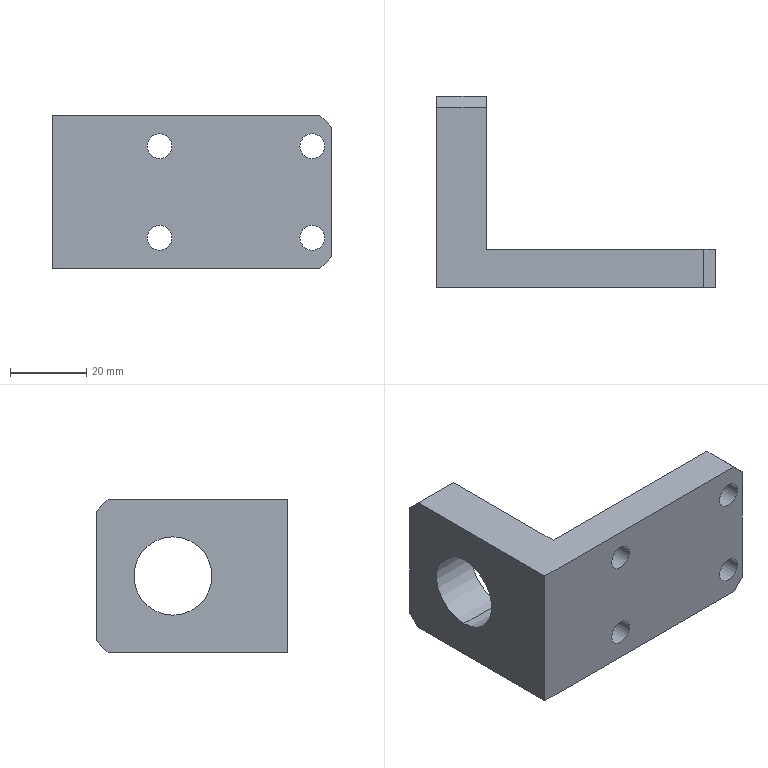Part | STEP file | 1 solid | 22 faces | box 73 x 50 x 40 mm | volume 44175 mm3 | plane 12 | cylinder 10 | commonest cylinder face diameters 6.5 x8 20.5 x2